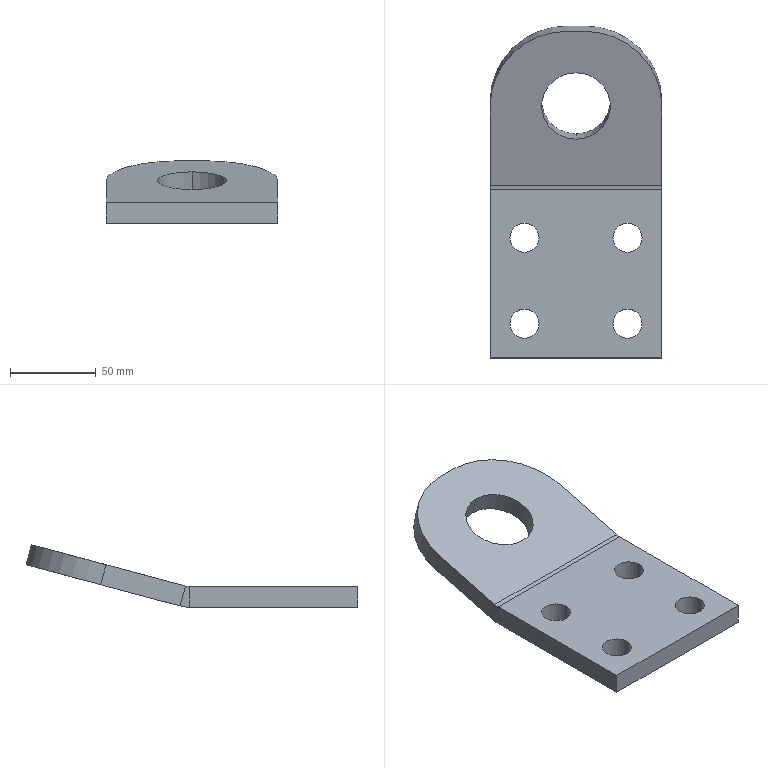Part | SolidWorks | 1 solid | 26 faces | box 100 x 193.34 x 36.386 mm | volume 197596 mm3 | cylinder 14 | plane 12 | commonest cylinder face diameters 17 x8 40 x2 90 x2 20 x1 44 x1
STEP:
#1=CARTESIAN_POINT('',(-38.5,-27.5,-12.));
#2=VERTEX_POINT('',#1);
#3=CARTESIAN_POINT('',(-21.5,-27.5,-12.));
#4=VERTEX_POINT('',#3);
#5=CARTESIAN_POINT('',(-30.,-27.5,-12.));
#6=DIRECTION('',(0.,0.,1.));
#7=DIRECTION('',(-1.,0.,0.));
#8=AXIS2_PLACEMENT_3D('',#5,#6,#7);
#9=CIRCLE('',#8,8.5);
#10=EDGE_CURVE('',#2,#4,#9,.T.);
#11=ORIENTED_EDGE('',*,*,#10,.F.);
#12=CARTESIAN_POINT('',(-38.5,-27.5,0.));
#13=VERTEX_POINT('',#12);
#14=CARTESIAN_POINT('',(-38.5,-27.5,-12.001));
#15=DIRECTION('',(0.,0.,1.));
#16=VECTOR('',#15,1000.);
#17=LINE('',#14,#16);
#18=EDGE_CURVE('',#2,#13,#17,.T.);
#19=ORIENTED_EDGE('',*,*,#18,.T.);
#20=CARTESIAN_POINT('',(-21.5,-27.5,0.));
#21=VERTEX_POINT('',#20);
#22=CARTESIAN_POINT('',(-30.,-27.5,0.));
#23=DIRECTION('',(0.,0.,1.));
#24=DIRECTION('',(1.,0.,0.));
#25=AXIS2_PLACEMENT_3D('',#22,#23,#24);
#26=CIRCLE('',#25,8.5);
#27=EDGE_CURVE('',#13,#21,#26,.T.);
#28=ORIENTED_EDGE('',*,*,#27,.T.);
#29=CARTESIAN_POINT('',(-21.5,-27.5,-12.001));
#30=DIRECTION('',(0.,0.,1.));
#31=VECTOR('',#30,1000.);
#32=LINE('',#29,#31);
#33=EDGE_CURVE('',#4,#21,#32,.T.);
#34=ORIENTED_EDGE('',*,*,#33,.F.);
#35=EDGE_LOOP('',(#11,#19,#28,#34));
#36=FACE_OUTER_BOUND('',#35,.T.);
#37=CARTESIAN_POINT('',(-30.,-27.5,-12.001));
#38=DIRECTION('',(0.,0.,1.));
#39=DIRECTION('',(1.,0.,0.));
#40=AXIS2_PLACEMENT_3D('',#37,#38,#39);
#41=CYLINDRICAL_SURFACE('',#40,8.5);
#42=ADVANCED_FACE('',(#36),#41,.F.);
#43=CARTESIAN_POINT('',(21.5,-27.5,-12.));
#44=VERTEX_POINT('',#43);
#45=CARTESIAN_POINT('',(38.5,-27.5,-12.));
#46=VERTEX_POINT('',#45);
#47=CARTESIAN_POINT('',(30.,-27.5,-12.));
#48=DIRECTION('',(0.,0.,1.));
#49=DIRECTION('',(-1.,0.,0.));
#50=AXIS2_PLACEMENT_3D('',#47,#48,#49);
#51=CIRCLE('',#50,8.5);
#52=EDGE_CURVE('',#44,#46,#51,.T.);
#53=ORIENTED_EDGE('',*,*,#52,.F.);
#54=CARTESIAN_POINT('',(21.5,-27.5,0.));
#55=VERTEX_POINT('',#54);
#56=CARTESIAN_POINT('',(21.5,-27.5,-12.001));
#57=DIRECTION('',(0.,0.,1.));
#58=VECTOR('',#57,1000.);
#59=LINE('',#56,#58);
#60=EDGE_CURVE('',#44,#55,#59,.T.);
#61=ORIENTED_EDGE('',*,*,#60,.T.);
#62=CARTESIAN_POINT('',(38.5,-27.5,0.));
#63=VERTEX_POINT('',#62);
#64=CARTESIAN_POINT('',(30.,-27.5,0.));
#65=DIRECTION('',(0.,0.,1.));
#66=DIRECTION('',(1.,0.,0.));
#67=AXIS2_PLACEMENT_3D('',#64,#65,#66);
#68=CIRCLE('',#67,8.5);
#69=EDGE_CURVE('',#55,#63,#68,.T.);
#70=ORIENTED_EDGE('',*,*,#69,.T.);
#71=CARTESIAN_POINT('',(38.5,-27.5,-12.001));
#72=DIRECTION('',(0.,0.,1.));
#73=VECTOR('',#72,1000.);
#74=LINE('',#71,#73);
#75=EDGE_CURVE('',#46,#63,#74,.T.);
#76=ORIENTED_EDGE('',*,*,#75,.F.);
#77=EDGE_LOOP('',(#53,#61,#70,#76));
#78=FACE_OUTER_BOUND('',#77,.T.);
#79=CARTESIAN_POINT('',(30.,-27.5,-12.001));
#80=DIRECTION('',(0.,0.,1.));
#81=DIRECTION('',(1.,0.,0.));
#82=AXIS2_PLACEMENT_3D('',#79,#80,#81);
#83=CYLINDRICAL_SURFACE('',#82,8.5);
#84=ADVANCED_FACE('',(#78),#83,.F.);
#85=CARTESIAN_POINT('',(21.5,-77.5,-12.));
#86=VERTEX_POINT('',#85);
#87=CARTESIAN_POINT('',(38.5,-77.5,-12.));
#88=VERTEX_POINT('',#87);
#89=CARTESIAN_POINT('',(30.,-77.5,-12.));
#90=DIRECTION('',(0.,0.,1.));
#91=DIRECTION('',(-1.,0.,0.));
#92=AXIS2_PLACEMENT_3D('',#89,#90,#91);
#93=CIRCLE('',#92,8.5);
#94=EDGE_CURVE('',#86,#88,#93,.T.);
#95=ORIENTED_EDGE('',*,*,#94,.F.);
#96=CARTESIAN_POINT('',(21.5,-77.5,0.));
#97=VERTEX_POINT('',#96);
#98=CARTESIAN_POINT('',(21.5,-77.5,-12.001));
#99=DIRECTION('',(0.,0.,1.));
#100=VECTOR('',#99,1000.);
#101=LINE('',#98,#100);
#102=EDGE_CURVE('',#86,#97,#101,.T.);
#103=ORIENTED_EDGE('',*,*,#102,.T.);
#104=CARTESIAN_POINT('',(38.5,-77.5,0.));
#105=VERTEX_POINT('',#104);
#106=CARTESIAN_POINT('',(30.,-77.5,0.));
#107=DIRECTION('',(0.,0.,1.));
#108=DIRECTION('',(1.,0.,0.));
#109=AXIS2_PLACEMENT_3D('',#106,#107,#108);
#110=CIRCLE('',#109,8.5);
#111=EDGE_CURVE('',#97,#105,#110,.T.);
#112=ORIENTED_EDGE('',*,*,#111,.T.);
#113=CARTESIAN_POINT('',(38.5,-77.5,-12.001));
#114=DIRECTION('',(0.,0.,1.));
#115=VECTOR('',#114,1000.);
#116=LINE('',#113,#115);
#117=EDGE_CURVE('',#88,#105,#116,.T.);
#118=ORIENTED_EDGE('',*,*,#117,.F.);
#119=EDGE_LOOP('',(#95,#103,#112,#118));
#120=FACE_OUTER_BOUND('',#119,.T.);
#121=CARTESIAN_POINT('',(30.,-77.5,-12.001));
#122=DIRECTION('',(0.,0.,1.));
#123=DIRECTION('',(1.,0.,0.));
#124=AXIS2_PLACEMENT_3D('',#121,#122,#123);
#125=CYLINDRICAL_SURFACE('',#124,8.5);
#126=ADVANCED_FACE('',(#120),#125,.F.);
#127=CARTESIAN_POINT('',(-38.5,-77.5,-12.));
#128=VERTEX_POINT('',#127);
#129=CARTESIAN_POINT('',(-21.5,-77.5,-12.));
#130=VERTEX_POINT('',#129);
#131=CARTESIAN_POINT('',(-30.,-77.5,-12.));
#132=DIRECTION('',(0.,0.,1.));
#133=DIRECTION('',(-1.,0.,0.));
#134=AXIS2_PLACEMENT_3D('',#131,#132,#133);
#135=CIRCLE('',#134,8.5);
#136=EDGE_CURVE('',#128,#130,#135,.T.);
#137=ORIENTED_EDGE('',*,*,#136,.F.);
#138=CARTESIAN_POINT('',(-38.5,-77.5,0.));
#139=VERTEX_POINT('',#138);
#140=CARTESIAN_POINT('',(-38.5,-77.5,-12.001));
#141=DIRECTION('',(0.,0.,1.));
#142=VECTOR('',#141,1000.);
#143=LINE('',#140,#142);
#144=EDGE_CURVE('',#128,#139,#143,.T.);
#145=ORIENTED_EDGE('',*,*,#144,.T.);
#146=CARTESIAN_POINT('',(-21.5,-77.5,0.));
#147=VERTEX_POINT('',#146);
#148=CARTESIAN_POINT('',(-30.,-77.5,0.));
#149=DIRECTION('',(0.,0.,1.));
#150=DIRECTION('',(1.,0.,0.));
#151=AXIS2_PLACEMENT_3D('',#148,#149,#150);
#152=CIRCLE('',#151,8.5);
#153=EDGE_CURVE('',#139,#147,#152,.T.);
#154=ORIENTED_EDGE('',*,*,#153,.T.);
#155=CARTESIAN_POINT('',(-21.5,-77.5,-12.001));
#156=DIRECTION('',(0.,0.,1.));
#157=VECTOR('',#156,1000.);
#158=LINE('',#155,#157);
#159=EDGE_CURVE('',#130,#147,#158,.T.);
#160=ORIENTED_EDGE('',*,*,#159,.F.);
#161=EDGE_LOOP('',(#137,#145,#154,#160));
#162=FACE_OUTER_BOUND('',#161,.T.);
#163=CARTESIAN_POINT('',(-30.,-77.5,-12.001));
#164=DIRECTION('',(0.,0.,1.));
#165=DIRECTION('',(1.,0.,0.));
#166=AXIS2_PLACEMENT_3D('',#163,#164,#165);
#167=CYLINDRICAL_SURFACE('',#166,8.5);
#168=ADVANCED_FACE('',(#162),#167,.F.);
#169=CARTESIAN_POINT('',(0.,68.586,17.916));
#170=VERTEX_POINT('',#169);
#171=CARTESIAN_POINT('',(0.,29.949,7.563));
#172=VERTEX_POINT('',#171);
#173=CARTESIAN_POINT('',(0.,49.267,12.74));
#174=DIRECTION('',(0.,-0.2588,0.9659));
#175=DIRECTION('',(0.,0.9659,0.2588));
#176=AXIS2_PLACEMENT_3D('',#173,#174,#175);
#177=CIRCLE('',#176,20.);
#178=EDGE_CURVE('',#170,#172,#177,.T.);
#179=ORIENTED_EDGE('',*,*,#178,.T.);
#180=CARTESIAN_POINT('',(0.,33.054,-4.028));
#181=VERTEX_POINT('',#180);
#182=CARTESIAN_POINT('',(0.,17.205,55.123));
#183=DIRECTION('',(0.,0.2588,-0.9659));
#184=VECTOR('',#183,1000.);
#185=LINE('',#182,#184);
#186=EDGE_CURVE('',#172,#181,#185,.T.);
#187=ORIENTED_EDGE('',*,*,#186,.T.);
#188=CARTESIAN_POINT('',(0.,71.691,6.325));
#189=VERTEX_POINT('',#188);
#190=CARTESIAN_POINT('',(0.,52.373,1.149));
#191=DIRECTION('',(0.,0.2588,-0.9659));
#192=DIRECTION('',(0.,0.9659,0.2588));
#193=AXIS2_PLACEMENT_3D('',#190,#191,#192);
#194=CIRCLE('',#193,20.);
#195=EDGE_CURVE('',#181,#189,#194,.T.);
#196=ORIENTED_EDGE('',*,*,#195,.T.);
#197=CARTESIAN_POINT('',(0.,55.842,65.476));
#198=DIRECTION('',(0.,0.2588,-0.9659));
#199=VECTOR('',#198,1000.);
#200=LINE('',#197,#199);
#201=EDGE_CURVE('',#170,#189,#200,.T.);
#202=ORIENTED_EDGE('',*,*,#201,.F.);
#203=EDGE_LOOP('',(#179,#187,#196,#202));
#204=FACE_OUTER_BOUND('',#203,.T.);
#205=CARTESIAN_POINT('',(0.,36.523,60.299));
#206=DIRECTION('',(0.,0.2588,-0.9659));
#207=DIRECTION('',(0.,0.9659,0.2588));
#208=AXIS2_PLACEMENT_3D('',#205,#206,#207);
#209=CYLINDRICAL_SURFACE('',#208,20.);
#210=ADVANCED_FACE('',(#204),#209,.F.);
#211=ORIENTED_EDGE('',*,*,#178,.F.);
#212=CARTESIAN_POINT('',(0.,49.267,12.74));
#213=DIRECTION('',(0.,-0.2588,0.9659));
#214=DIRECTION('',(0.,0.9659,0.2588));
#215=AXIS2_PLACEMENT_3D('',#212,#213,#214);
#216=CIRCLE('',#215,20.);
#217=EDGE_CURVE('',#172,#170,#216,.T.);
#218=ORIENTED_EDGE('',*,*,#217,.F.);
#219=EDGE_LOOP('',(#211,#218));
#220=FACE_BOUND('',#219,.T.);
#221=CARTESIAN_POINT('',(5.,92.734,24.386));
#222=VERTEX_POINT('',#221);
#223=CARTESIAN_POINT('',(-5.,92.734,24.386));
#224=VERTEX_POINT('',#223);
#225=CARTESIAN_POINT('',(-50.,92.734,24.386));
#226=DIRECTION('',(-1.,0.,0.));
#227=VECTOR('',#226,1000.);
#228=LINE('',#225,#227);
#229=EDGE_CURVE('',#222,#224,#228,.T.);
#230=ORIENTED_EDGE('',*,*,#229,.T.);
#231=CARTESIAN_POINT('',(-50.,49.267,12.74));
#232=VERTEX_POINT('',#231);
#233=CARTESIAN_POINT('',(-5.,49.267,12.74));
#234=DIRECTION('',(0.,-0.2588,0.9659));
#235=DIRECTION('',(0.,0.9659,0.2588));
#236=AXIS2_PLACEMENT_3D('',#233,#234,#235);
#237=CIRCLE('',#236,45.);
#238=EDGE_CURVE('',#224,#232,#237,.T.);
#239=ORIENTED_EDGE('',*,*,#238,.T.);
#240=CARTESIAN_POINT('',(-50.,2.994,0.3407));
#241=VERTEX_POINT('',#240);
#242=CARTESIAN_POINT('',(-50.,-95.622,-26.083));
#243=DIRECTION('',(0.,-0.9659,-0.2588));
#244=VECTOR('',#243,1000.);
#245=LINE('',#242,#244);
#246=EDGE_CURVE('',#232,#241,#245,.T.);
#247=ORIENTED_EDGE('',*,*,#246,.T.);
#248=CARTESIAN_POINT('',(50.,2.994,0.3407));
#249=VERTEX_POINT('',#248);
#250=CARTESIAN_POINT('',(0.,2.994,0.3407));
#251=DIRECTION('',(1.,0.,0.));
#252=VECTOR('',#251,1000.);
#253=LINE('',#250,#252);
#254=EDGE_CURVE('',#241,#249,#253,.T.);
#255=ORIENTED_EDGE('',*,*,#254,.T.);
#256=CARTESIAN_POINT('',(50.,49.267,12.74));
#257=VERTEX_POINT('',#256);
#258=CARTESIAN_POINT('',(50.,-95.622,-26.083));
#259=DIRECTION('',(0.,0.9659,0.2588));
#260=VECTOR('',#259,1000.);
#261=LINE('',#258,#260);
#262=EDGE_CURVE('',#249,#257,#261,.T.);
#263=ORIENTED_EDGE('',*,*,#262,.T.);
#264=CARTESIAN_POINT('',(5.,49.267,12.74));
#265=DIRECTION('',(0.,-0.2588,0.9659));
#266=DIRECTION('',(0.,0.9659,0.2588));
#267=AXIS2_PLACEMENT_3D('',#264,#265,#266);
#268=CIRCLE('',#267,45.);
#269=EDGE_CURVE('',#257,#222,#268,.T.);
#270=ORIENTED_EDGE('',*,*,#269,.T.);
#271=EDGE_LOOP('',(#230,#239,#247,#255,#263,#270));
#272=FACE_OUTER_BOUND('',#271,.T.);
#273=CARTESIAN_POINT('',(0.,-1.444,-0.8484));
#274=DIRECTION('',(0.,0.2588,-0.9659));
#275=DIRECTION('',(-1.,0.,0.));
#276=AXIS2_PLACEMENT_3D('',#273,#274,#275);
#277=PLANE('',#276);
#278=ADVANCED_FACE('',(#220,#272),#277,.F.);
#279=CARTESIAN_POINT('',(50.,6.1,-11.25));
#280=VERTEX_POINT('',#279);
#281=CARTESIAN_POINT('',(50.,52.373,1.149));
#282=VERTEX_POINT('',#281);
#283=CARTESIAN_POINT('',(50.,-92.516,-37.674));
#284=DIRECTION('',(0.,0.9659,0.2588));
#285=VECTOR('',#284,1000.);
#286=LINE('',#283,#285);
#287=EDGE_CURVE('',#280,#282,#286,.T.);
#288=ORIENTED_EDGE('',*,*,#287,.T.);
#289=CARTESIAN_POINT('',(50.,52.373,1.149));
#290=DIRECTION('',(0.,-0.2588,0.9659));
#291=VECTOR('',#290,1000.);
#292=LINE('',#289,#291);
#293=EDGE_CURVE('',#282,#257,#292,.T.);
#294=ORIENTED_EDGE('',*,*,#293,.T.);
#295=ORIENTED_EDGE('',*,*,#262,.F.);
#296=CARTESIAN_POINT('',(50.,6.1,-11.25));
#297=DIRECTION('',(0.,-0.2588,0.9659));
#298=VECTOR('',#297,1000.);
#299=LINE('',#296,#298);
#300=EDGE_CURVE('',#280,#249,#299,.T.);
#301=ORIENTED_EDGE('',*,*,#300,.F.);
#302=EDGE_LOOP('',(#288,#294,#295,#301));
#303=FACE_OUTER_BOUND('',#302,.T.);
#304=CARTESIAN_POINT('',(50.,-92.516,-37.674));
#305=DIRECTION('',(1.,0.,0.));
#306=DIRECTION('',(0.,0.2588,-0.9659));
#307=AXIS2_PLACEMENT_3D('',#304,#305,#306);
#308=PLANE('',#307);
#309=ADVANCED_FACE('',(#303),#308,.T.);
#310=ORIENTED_EDGE('',*,*,#246,.F.);
#311=CARTESIAN_POINT('',(-50.,52.373,1.149));
#312=VERTEX_POINT('',#311);
#313=CARTESIAN_POINT('',(-50.,52.373,1.149));
#314=DIRECTION('',(0.,0.2588,-0.9659));
#315=VECTOR('',#314,1000.);
#316=LINE('',#313,#315);
#317=EDGE_CURVE('',#232,#312,#316,.T.);
#318=ORIENTED_EDGE('',*,*,#317,.T.);
#319=CARTESIAN_POINT('',(-50.,6.1,-11.25));
#320=VERTEX_POINT('',#319);
#321=CARTESIAN_POINT('',(-50.,-92.516,-37.674));
#322=DIRECTION('',(0.,-0.9659,-0.2588));
#323=VECTOR('',#322,1000.);
#324=LINE('',#321,#323);
#325=EDGE_CURVE('',#312,#320,#324,.T.);
#326=ORIENTED_EDGE('',*,*,#325,.T.);
#327=CARTESIAN_POINT('',(-50.,6.1,-11.25));
#328=DIRECTION('',(0.,0.2588,-0.9659));
#329=VECTOR('',#328,1000.);
#330=LINE('',#327,#329);
#331=EDGE_CURVE('',#241,#320,#330,.T.);
#332=ORIENTED_EDGE('',*,*,#331,.F.);
#333=EDGE_LOOP('',(#310,#318,#326,#332));
#334=FACE_OUTER_BOUND('',#333,.T.);
#335=CARTESIAN_POINT('',(-50.,-92.516,-37.674));
#336=DIRECTION('',(-1.,0.,0.));
#337=DIRECTION('',(0.,-0.2588,0.9659));
#338=AXIS2_PLACEMENT_3D('',#335,#336,#337);
#339=PLANE('',#338);
#340=ADVANCED_FACE('',(#334),#339,.T.);
#341=CARTESIAN_POINT('',(5.,95.84,12.795));
#342=VERTEX_POINT('',#341);
#343=CARTESIAN_POINT('',(-5.,95.84,12.795));
#344=VERTEX_POINT('',#343);
#345=CARTESIAN_POINT('',(-50.,95.84,12.795));
#346=DIRECTION('',(-1.,0.,0.));
#347=VECTOR('',#346,1000.);
#348=LINE('',#345,#347);
#349=EDGE_CURVE('',#342,#344,#348,.T.);
#350=ORIENTED_EDGE('',*,*,#349,.T.);
#351=CARTESIAN_POINT('',(-5.,95.84,12.795));
#352=DIRECTION('',(0.,-0.2588,0.9659));
#353=VECTOR('',#352,1000.);
#354=LINE('',#351,#353);
#355=EDGE_CURVE('',#344,#224,#354,.T.);
#356=ORIENTED_EDGE('',*,*,#355,.T.);
#357=ORIENTED_EDGE('',*,*,#229,.F.);
#358=CARTESIAN_POINT('',(5.,95.84,12.795));
#359=DIRECTION('',(0.,0.2588,-0.9659));
#360=VECTOR('',#359,1000.);
#361=LINE('',#358,#360);
#362=EDGE_CURVE('',#222,#342,#361,.T.);
#363=ORIENTED_EDGE('',*,*,#362,.T.);
#364=EDGE_LOOP('',(#350,#356,#357,#363));
#365=FACE_OUTER_BOUND('',#364,.T.);
#366=CARTESIAN_POINT('',(-50.,95.84,12.795));
#367=DIRECTION('',(0.,0.9659,0.2588));
#368=DIRECTION('',(0.,-0.2588,0.9659));
#369=AXIS2_PLACEMENT_3D('',#366,#367,#368);
#370=PLANE('',#369);
#371=ADVANCED_FACE('',(#365),#370,.T.);
#372=CARTESIAN_POINT('',(0.,52.373,1.149));
#373=DIRECTION('',(0.,0.2588,-0.9659));
#374=DIRECTION('',(0.,0.9659,0.2588));
#375=AXIS2_PLACEMENT_3D('',#372,#373,#374);
#376=CIRCLE('',#375,20.);
#377=EDGE_CURVE('',#189,#181,#376,.T.);
#378=ORIENTED_EDGE('',*,*,#377,.F.);
#379=ORIENTED_EDGE('',*,*,#195,.F.);
#380=EDGE_LOOP('',(#378,#379));
#381=FACE_BOUND('',#380,.T.);
#382=ORIENTED_EDGE('',*,*,#325,.F.);
#383=CARTESIAN_POINT('',(-5.,52.373,1.149));
#384=DIRECTION('',(0.,0.2588,-0.9659));
#385=DIRECTION('',(0.,0.9659,0.2588));
#386=AXIS2_PLACEMENT_3D('',#383,#384,#385);
#387=CIRCLE('',#386,45.);
#388=EDGE_CURVE('',#312,#344,#387,.T.);
#389=ORIENTED_EDGE('',*,*,#388,.T.);
#390=ORIENTED_EDGE('',*,*,#349,.F.);
#391=CARTESIAN_POINT('',(5.,52.373,1.149));
#392=DIRECTION('',(0.,0.2588,-0.9659));
#393=DIRECTION('',(0.,0.9659,0.2588));
#394=AXIS2_PLACEMENT_3D('',#391,#392,#393);
#395=CIRCLE('',#394,45.);
#396=EDGE_CURVE('',#342,#282,#395,.T.);
#397=ORIENTED_EDGE('',*,*,#396,.T.);
#398=ORIENTED_EDGE('',*,*,#287,.F.);
#399=CARTESIAN_POINT('',(0.,6.1,-11.25));
#400=DIRECTION('',(1.,0.,0.));
#401=VECTOR('',#400,1000.);
#402=LINE('',#399,#401);
#403=EDGE_CURVE('',#320,#280,#402,.T.);
#404=ORIENTED_EDGE('',*,*,#403,.F.);
#405=EDGE_LOOP('',(#382,#389,#390,#397,#398,#404));
#406=FACE_OUTER_BOUND('',#405,.T.);
#407=CARTESIAN_POINT('',(0.,1.662,-12.439));
#408=DIRECTION('',(0.,0.2588,-0.9659));
#409=DIRECTION('',(-1.,0.,0.));
#410=AXIS2_PLACEMENT_3D('',#407,#408,#409);
#411=PLANE('',#410);
#412=ADVANCED_FACE('',(#381,#406),#411,.T.);
#413=CARTESIAN_POINT('',(-50.,-97.5,0.));
#414=VERTEX_POINT('',#413);
#415=CARTESIAN_POINT('',(50.,-97.5,0.));
#416=VERTEX_POINT('',#415);
#417=CARTESIAN_POINT('',(-50.,-97.5,0.));
#418=DIRECTION('',(1.,0.,0.));
#419=VECTOR('',#418,1000.);
#420=LINE('',#417,#419);
#421=EDGE_CURVE('',#414,#416,#420,.T.);
#422=ORIENTED_EDGE('',*,*,#421,.F.);
#423=CARTESIAN_POINT('',(-50.,-97.5,-12.));
#424=VERTEX_POINT('',#423);
#425=CARTESIAN_POINT('',(-50.,-97.5,-12.));
#426=DIRECTION('',(0.,0.,1.));
#427=VECTOR('',#426,1000.);
#428=LINE('',#425,#427);
#429=EDGE_CURVE('',#424,#414,#428,.T.);
#430=ORIENTED_EDGE('',*,*,#429,.F.);
#431=CARTESIAN_POINT('',(50.,-97.5,-12.));
#432=VERTEX_POINT('',#431);
#433=CARTESIAN_POINT('',(-50.,-97.5,-12.));
#434=DIRECTION('',(1.,0.,0.));
#435=VECTOR('',#434,1000.);
#436=LINE('',#433,#435);
#437=EDGE_CURVE('',#424,#432,#436,.T.);
#438=ORIENTED_EDGE('',*,*,#437,.T.);
#439=CARTESIAN_POINT('',(50.,-97.5,-12.));
#440=DIRECTION('',(0.,0.,1.));
#441=VECTOR('',#440,1000.);
#442=LINE('',#439,#441);
#443=EDGE_CURVE('',#432,#416,#442,.T.);
#444=ORIENTED_EDGE('',*,*,#443,.T.);
#445=EDGE_LOOP('',(#422,#430,#438,#444));
#446=FACE_OUTER_BOUND('',#445,.T.);
#447=CARTESIAN_POINT('',(-50.,-97.5,-12.));
#448=DIRECTION('',(0.,-1.,0.));
#449=DIRECTION('',(0.,0.,-1.));
#450=AXIS2_PLACEMENT_3D('',#447,#448,#449);
#451=PLANE('',#450);
#452=ADVANCED_FACE('',(#446),#451,.T.);
#453=CARTESIAN_POINT('',(-30.,-27.5,-12.));
#454=DIRECTION('',(0.,0.,1.));
#455=DIRECTION('',(-1.,0.,0.));
#456=AXIS2_PLACEMENT_3D('',#453,#454,#455);
#457=CIRCLE('',#456,8.5);
#458=EDGE_CURVE('',#4,#2,#457,.T.);
#459=ORIENTED_EDGE('',*,*,#458,.T.);
#460=ORIENTED_EDGE('',*,*,#10,.T.);
#461=EDGE_LOOP('',(#459,#460));
#462=FACE_BOUND('',#461,.T.);
#463=CARTESIAN_POINT('',(30.,-27.5,-12.));
#464=DIRECTION('',(0.,0.,1.));
#465=DIRECTION('',(-1.,0.,0.));
#466=AXIS2_PLACEMENT_3D('',#463,#464,#465);
#467=CIRCLE('',#466,8.5);
#468=EDGE_CURVE('',#46,#44,#467,.T.);
#469=ORIENTED_EDGE('',*,*,#468,.T.);
#470=ORIENTED_EDGE('',*,*,#52,.T.);
#471=EDGE_LOOP('',(#469,#470));
#472=FACE_BOUND('',#471,.T.);
#473=CARTESIAN_POINT('',(30.,-77.5,-12.));
#474=DIRECTION('',(0.,0.,1.));
#475=DIRECTION('',(-1.,0.,0.));
#476=AXIS2_PLACEMENT_3D('',#473,#474,#475);
#477=CIRCLE('',#476,8.5);
#478=EDGE_CURVE('',#88,#86,#477,.T.);
#479=ORIENTED_EDGE('',*,*,#478,.T.);
#480=ORIENTED_EDGE('',*,*,#94,.T.);
#481=EDGE_LOOP('',(#479,#480));
#482=FACE_BOUND('',#481,.T.);
#483=CARTESIAN_POINT('',(-30.,-77.5,-12.));
#484=DIRECTION('',(0.,0.,1.));
#485=DIRECTION('',(-1.,0.,0.));
#486=AXIS2_PLACEMENT_3D('',#483,#484,#485);
#487=CIRCLE('',#486,8.5);
#488=EDGE_CURVE('',#130,#128,#487,.T.);
#489=ORIENTED_EDGE('',*,*,#488,.T.);
#490=ORIENTED_EDGE('',*,*,#136,.T.);
#491=EDGE_LOOP('',(#489,#490));
#492=FACE_BOUND('',#491,.T.);
#493=CARTESIAN_POINT('',(-50.,0.4056,-12.));
#494=VERTEX_POINT('',#493);
#495=CARTESIAN_POINT('',(-50.,-97.5,-12.));
#496=DIRECTION('',(0.,-1.,0.));
#497=VECTOR('',#496,1000.);
#498=LINE('',#495,#497);
#499=EDGE_CURVE('',#494,#424,#498,.T.);
#500=ORIENTED_EDGE('',*,*,#499,.F.);
#501=CARTESIAN_POINT('',(50.,0.4056,-12.));
#502=VERTEX_POINT('',#501);
#503=CARTESIAN_POINT('',(0.,0.4056,-12.));
#504=DIRECTION('',(1.,0.,0.));
#505=VECTOR('',#504,1000.);
#506=LINE('',#503,#505);
#507=EDGE_CURVE('',#494,#502,#506,.T.);
#508=ORIENTED_EDGE('',*,*,#507,.T.);
#509=CARTESIAN_POINT('',(50.,-97.5,-12.));
#510=DIRECTION('',(0.,1.,0.));
#511=VECTOR('',#510,1000.);
#512=LINE('',#509,#511);
#513=EDGE_CURVE('',#432,#502,#512,.T.);
#514=ORIENTED_EDGE('',*,*,#513,.F.);
#515=ORIENTED_EDGE('',*,*,#437,.F.);
#516=EDGE_LOOP('',(#500,#508,#514,#515));
#517=FACE_OUTER_BOUND('',#516,.T.);
#518=CARTESIAN_POINT('',(0.,0.,-12.));
#519=DIRECTION('',(0.,0.,-1.));
#520=DIRECTION('',(-1.,0.,0.));
#521=AXIS2_PLACEMENT_3D('',#518,#519,#520);
#522=PLANE('',#521);
#523=ADVANCED_FACE('',(#462,#472,#482,#492,#517),#522,.T.);
#524=ORIENTED_EDGE('',*,*,#513,.T.);
#525=CARTESIAN_POINT('',(50.,0.4056,0.));
#526=VERTEX_POINT('',#525);
#527=CARTESIAN_POINT('',(50.,0.4056,-12.));
#528=DIRECTION('',(0.,0.,1.));
#529=VECTOR('',#528,1000.);
#530=LINE('',#527,#529);
#531=EDGE_CURVE('',#502,#526,#530,.T.);
#532=ORIENTED_EDGE('',*,*,#531,.T.);
#533=CARTESIAN_POINT('',(50.,-97.5,0.));
#534=DIRECTION('',(0.,1.,0.));
#535=VECTOR('',#534,1000.);
#536=LINE('',#533,#535);
#537=EDGE_CURVE('',#416,#526,#536,.T.);
#538=ORIENTED_EDGE('',*,*,#537,.F.);
#539=ORIENTED_EDGE('',*,*,#443,.F.);
#540=EDGE_LOOP('',(#524,#532,#538,#539));
#541=FACE_OUTER_BOUND('',#540,.T.);
#542=CARTESIAN_POINT('',(50.,-97.5,-12.));
#543=DIRECTION('',(1.,0.,0.));
#544=DIRECTION('',(0.,0.,-1.));
#545=AXIS2_PLACEMENT_3D('',#542,#543,#544);
#546=PLANE('',#545);
#547=ADVANCED_FACE('',(#541),#546,.T.);
#548=CARTESIAN_POINT('',(-30.,-27.5,0.));
#549=DIRECTION('',(0.,0.,1.));
#550=DIRECTION('',(1.,0.,0.));
#551=AXIS2_PLACEMENT_3D('',#548,#549,#550);
#552=CIRCLE('',#551,8.5);
#553=EDGE_CURVE('',#21,#13,#552,.T.);
#554=ORIENTED_EDGE('',*,*,#553,.F.);
#555=ORIENTED_EDGE('',*,*,#27,.F.);
#556=EDGE_LOOP('',(#554,#555));
#557=FACE_BOUND('',#556,.T.);
#558=CARTESIAN_POINT('',(30.,-27.5,0.));
#559=DIRECTION('',(0.,0.,1.));
#560=DIRECTION('',(1.,0.,0.));
#561=AXIS2_PLACEMENT_3D('',#558,#559,#560);
#562=CIRCLE('',#561,8.5);
#563=EDGE_CURVE('',#63,#55,#562,.T.);
#564=ORIENTED_EDGE('',*,*,#563,.F.);
#565=ORIENTED_EDGE('',*,*,#69,.F.);
#566=EDGE_LOOP('',(#564,#565));
#567=FACE_BOUND('',#566,.T.);
#568=CARTESIAN_POINT('',(30.,-77.5,0.));
#569=DIRECTION('',(0.,0.,1.));
#570=DIRECTION('',(1.,0.,0.));
#571=AXIS2_PLACEMENT_3D('',#568,#569,#570);
#572=CIRCLE('',#571,8.5);
#573=EDGE_CURVE('',#105,#97,#572,.T.);
#574=ORIENTED_EDGE('',*,*,#573,.F.);
#575=ORIENTED_EDGE('',*,*,#111,.F.);
#576=EDGE_LOOP('',(#574,#575));
#577=FACE_BOUND('',#576,.T.);
#578=CARTESIAN_POINT('',(-30.,-77.5,0.));
#579=DIRECTION('',(0.,0.,1.));
#580=DIRECTION('',(1.,0.,0.));
#581=AXIS2_PLACEMENT_3D('',#578,#579,#580);
#582=CIRCLE('',#581,8.5);
#583=EDGE_CURVE('',#147,#139,#582,.T.);
#584=ORIENTED_EDGE('',*,*,#583,.F.);
#585=ORIENTED_EDGE('',*,*,#153,.F.);
#586=EDGE_LOOP('',(#584,#585));
#587=FACE_BOUND('',#586,.T.);
#588=CARTESIAN_POINT('',(-50.,0.4056,0.));
#589=VERTEX_POINT('',#588);
#590=CARTESIAN_POINT('',(0.,0.4056,0.));
#591=DIRECTION('',(1.,0.,0.));
#592=VECTOR('',#591,1000.);
#593=LINE('',#590,#592);
#594=EDGE_CURVE('',#589,#526,#593,.T.);
#595=ORIENTED_EDGE('',*,*,#594,.F.);
#596=CARTESIAN_POINT('',(-50.,-97.5,0.));
#597=DIRECTION('',(0.,-1.,0.));
#598=VECTOR('',#597,1000.);
#599=LINE('',#596,#598);
#600=EDGE_CURVE('',#589,#414,#599,.T.);
#601=ORIENTED_EDGE('',*,*,#600,.T.);
#602=ORIENTED_EDGE('',*,*,#421,.T.);
#603=ORIENTED_EDGE('',*,*,#537,.T.);
#604=EDGE_LOOP('',(#595,#601,#602,#603));
#605=FACE_OUTER_BOUND('',#604,.T.);
#606=CARTESIAN_POINT('',(0.,0.,0.));
#607=DIRECTION('',(0.,0.,-1.));
#608=DIRECTION('',(-1.,0.,0.));
#609=AXIS2_PLACEMENT_3D('',#606,#607,#608);
#610=PLANE('',#609);
#611=ADVANCED_FACE('',(#557,#567,#577,#587,#605),#610,.F.);
#612=ORIENTED_EDGE('',*,*,#600,.F.);
#613=CARTESIAN_POINT('',(-50.,0.4056,-12.));
#614=DIRECTION('',(0.,0.,-1.));
#615=VECTOR('',#614,1000.);
#616=LINE('',#613,#615);
#617=EDGE_CURVE('',#589,#494,#616,.T.);
#618=ORIENTED_EDGE('',*,*,#617,.T.);
#619=ORIENTED_EDGE('',*,*,#499,.T.);
#620=ORIENTED_EDGE('',*,*,#429,.T.);
#621=EDGE_LOOP('',(#612,#618,#619,#620));
#622=FACE_OUTER_BOUND('',#621,.T.);
#623=CARTESIAN_POINT('',(-50.,-97.5,-12.));
#624=DIRECTION('',(-1.,0.,0.));
#625=DIRECTION('',(0.,0.,1.));
#626=AXIS2_PLACEMENT_3D('',#623,#624,#625);
#627=PLANE('',#626);
#628=ADVANCED_FACE('',(#622),#627,.T.);
#629=ORIENTED_EDGE('',*,*,#617,.F.);
#630=CARTESIAN_POINT('',(-50.,0.4056,10.));
#631=DIRECTION('',(1.,0.,0.));
#632=DIRECTION('',(0.,0.,-1.));
#633=AXIS2_PLACEMENT_3D('',#630,#631,#632);
#634=CIRCLE('',#633,10.);
#635=EDGE_CURVE('',#589,#241,#634,.T.);
#636=ORIENTED_EDGE('',*,*,#635,.T.);
#637=ORIENTED_EDGE('',*,*,#331,.T.);
#638=CARTESIAN_POINT('',(-50.,0.4056,10.));
#639=DIRECTION('',(1.,0.,0.));
#640=DIRECTION('',(0.,0.,1.));
#641=AXIS2_PLACEMENT_3D('',#638,#639,#640);
#642=CIRCLE('',#641,22.);
#643=EDGE_CURVE('',#494,#320,#642,.T.);
#644=ORIENTED_EDGE('',*,*,#643,.F.);
#645=EDGE_LOOP('',(#629,#636,#637,#644));
#646=FACE_OUTER_BOUND('',#645,.T.);
#647=CARTESIAN_POINT('',(-50.,0.4056,10.));
#648=DIRECTION('',(-1.,0.,0.));
#649=DIRECTION('',(0.,0.,1.));
#650=AXIS2_PLACEMENT_3D('',#647,#648,#649);
#651=PLANE('',#650);
#652=ADVANCED_FACE('',(#646),#651,.T.);
#653=CARTESIAN_POINT('',(50.,0.4056,10.));
#654=DIRECTION('',(-1.,0.,0.));
#655=DIRECTION('',(0.,0.,-1.));
#656=AXIS2_PLACEMENT_3D('',#653,#654,#655);
#657=CIRCLE('',#656,10.);
#658=EDGE_CURVE('',#249,#526,#657,.T.);
#659=ORIENTED_EDGE('',*,*,#658,.T.);
#660=ORIENTED_EDGE('',*,*,#531,.F.);
#661=CARTESIAN_POINT('',(50.,0.4056,10.));
#662=DIRECTION('',(-1.,0.,0.));
#663=DIRECTION('',(0.,0.,-1.));
#664=AXIS2_PLACEMENT_3D('',#661,#662,#663);
#665=CIRCLE('',#664,22.);
#666=EDGE_CURVE('',#280,#502,#665,.T.);
#667=ORIENTED_EDGE('',*,*,#666,.F.);
#668=ORIENTED_EDGE('',*,*,#300,.T.);
#669=EDGE_LOOP('',(#659,#660,#667,#668));
#670=FACE_OUTER_BOUND('',#669,.T.);
#671=CARTESIAN_POINT('',(50.,0.4056,10.));
#672=DIRECTION('',(1.,0.,0.));
#673=DIRECTION('',(0.,0.,-1.));
#674=AXIS2_PLACEMENT_3D('',#671,#672,#673);
#675=PLANE('',#674);
#676=ADVANCED_FACE('',(#670),#675,.T.);
#677=ORIENTED_EDGE('',*,*,#403,.T.);
#678=ORIENTED_EDGE('',*,*,#666,.T.);
#679=ORIENTED_EDGE('',*,*,#507,.F.);
#680=ORIENTED_EDGE('',*,*,#643,.T.);
#681=EDGE_LOOP('',(#677,#678,#679,#680));
#682=FACE_OUTER_BOUND('',#681,.T.);
#683=CARTESIAN_POINT('',(-100.804,0.4056,10.));
#684=DIRECTION('',(1.,0.,0.));
#685=DIRECTION('',(0.,0.,-1.));
#686=AXIS2_PLACEMENT_3D('',#683,#684,#685);
#687=CYLINDRICAL_SURFACE('',#686,22.);
#688=ADVANCED_FACE('',(#682),#687,.T.);
#689=ORIENTED_EDGE('',*,*,#254,.F.);
#690=ORIENTED_EDGE('',*,*,#635,.F.);
#691=ORIENTED_EDGE('',*,*,#594,.T.);
#692=ORIENTED_EDGE('',*,*,#658,.F.);
#693=EDGE_LOOP('',(#689,#690,#691,#692));
#694=FACE_OUTER_BOUND('',#693,.T.);
#695=CARTESIAN_POINT('',(-100.804,0.4056,10.));
#696=DIRECTION('',(1.,0.,0.));
#697=DIRECTION('',(0.,0.,-1.));
#698=AXIS2_PLACEMENT_3D('',#695,#696,#697);
#699=CYLINDRICAL_SURFACE('',#698,10.);
#700=ADVANCED_FACE('',(#694),#699,.F.);
#701=ORIENTED_EDGE('',*,*,#186,.F.);
#702=ORIENTED_EDGE('',*,*,#217,.T.);
#703=ORIENTED_EDGE('',*,*,#201,.T.);
#704=ORIENTED_EDGE('',*,*,#377,.T.);
#705=EDGE_LOOP('',(#701,#702,#703,#704));
#706=FACE_OUTER_BOUND('',#705,.T.);
#707=CARTESIAN_POINT('',(0.,36.523,60.299));
#708=DIRECTION('',(0.,0.2588,-0.9659));
#709=DIRECTION('',(0.,0.9659,0.2588));
#710=AXIS2_PLACEMENT_3D('',#707,#708,#709);
#711=CYLINDRICAL_SURFACE('',#710,20.);
#712=ADVANCED_FACE('',(#706),#711,.F.);
#713=ORIENTED_EDGE('',*,*,#388,.F.);
#714=ORIENTED_EDGE('',*,*,#317,.F.);
#715=ORIENTED_EDGE('',*,*,#238,.F.);
#716=ORIENTED_EDGE('',*,*,#355,.F.);
#717=EDGE_LOOP('',(#713,#714,#715,#716));
#718=FACE_OUTER_BOUND('',#717,.T.);
#719=CARTESIAN_POINT('',(-5.,52.373,1.149));
#720=DIRECTION('',(0.,-0.2588,0.9659));
#721=DIRECTION('',(0.,-0.9659,-0.2588));
#722=AXIS2_PLACEMENT_3D('',#719,#720,#721);
#723=CYLINDRICAL_SURFACE('',#722,45.);
#724=ADVANCED_FACE('',(#718),#723,.T.);
#725=ORIENTED_EDGE('',*,*,#396,.F.);
#726=ORIENTED_EDGE('',*,*,#362,.F.);
#727=ORIENTED_EDGE('',*,*,#269,.F.);
#728=ORIENTED_EDGE('',*,*,#293,.F.);
#729=EDGE_LOOP('',(#725,#726,#727,#728));
#730=FACE_OUTER_BOUND('',#729,.T.);
#731=CARTESIAN_POINT('',(5.,52.373,1.149));
#732=DIRECTION('',(0.,-0.2588,0.9659));
#733=DIRECTION('',(0.,-0.9659,-0.2588));
#734=AXIS2_PLACEMENT_3D('',#731,#732,#733);
#735=CYLINDRICAL_SURFACE('',#734,45.);
#736=ADVANCED_FACE('',(#730),#735,.T.);
#737=ORIENTED_EDGE('',*,*,#144,.F.);
#738=ORIENTED_EDGE('',*,*,#488,.F.);
#739=ORIENTED_EDGE('',*,*,#159,.T.);
#740=ORIENTED_EDGE('',*,*,#583,.T.);
#741=EDGE_LOOP('',(#737,#738,#739,#740));
#742=FACE_OUTER_BOUND('',#741,.T.);
#743=CARTESIAN_POINT('',(-30.,-77.5,-12.001));
#744=DIRECTION('',(0.,0.,1.));
#745=DIRECTION('',(1.,0.,0.));
#746=AXIS2_PLACEMENT_3D('',#743,#744,#745);
#747=CYLINDRICAL_SURFACE('',#746,8.5);
#748=ADVANCED_FACE('',(#742),#747,.F.);
#749=ORIENTED_EDGE('',*,*,#102,.F.);
#750=ORIENTED_EDGE('',*,*,#478,.F.);
#751=ORIENTED_EDGE('',*,*,#117,.T.);
#752=ORIENTED_EDGE('',*,*,#573,.T.);
#753=EDGE_LOOP('',(#749,#750,#751,#752));
#754=FACE_OUTER_BOUND('',#753,.T.);
#755=CARTESIAN_POINT('',(30.,-77.5,-12.001));
#756=DIRECTION('',(0.,0.,1.));
#757=DIRECTION('',(1.,0.,0.));
#758=AXIS2_PLACEMENT_3D('',#755,#756,#757);
#759=CYLINDRICAL_SURFACE('',#758,8.5);
#760=ADVANCED_FACE('',(#754),#759,.F.);
#761=ORIENTED_EDGE('',*,*,#60,.F.);
#762=ORIENTED_EDGE('',*,*,#468,.F.);
#763=ORIENTED_EDGE('',*,*,#75,.T.);
#764=ORIENTED_EDGE('',*,*,#563,.T.);
#765=EDGE_LOOP('',(#761,#762,#763,#764));
#766=FACE_OUTER_BOUND('',#765,.T.);
#767=CARTESIAN_POINT('',(30.,-27.5,-12.001));
#768=DIRECTION('',(0.,0.,1.));
#769=DIRECTION('',(1.,0.,0.));
#770=AXIS2_PLACEMENT_3D('',#767,#768,#769);
#771=CYLINDRICAL_SURFACE('',#770,8.5);
#772=ADVANCED_FACE('',(#766),#771,.F.);
#773=ORIENTED_EDGE('',*,*,#18,.F.);
#774=ORIENTED_EDGE('',*,*,#458,.F.);
#775=ORIENTED_EDGE('',*,*,#33,.T.);
#776=ORIENTED_EDGE('',*,*,#553,.T.);
#777=EDGE_LOOP('',(#773,#774,#775,#776));
#778=FACE_OUTER_BOUND('',#777,.T.);
#779=CARTESIAN_POINT('',(-30.,-27.5,-12.001));
#780=DIRECTION('',(0.,0.,1.));
#781=DIRECTION('',(1.,0.,0.));
#782=AXIS2_PLACEMENT_3D('',#779,#780,#781);
#783=CYLINDRICAL_SURFACE('',#782,8.5);
#784=ADVANCED_FACE('',(#778),#783,.F.);
#785=CLOSED_SHELL('',(#42,#84,#126,#168,#210,#278,#309,#340,#371,#412,#452,#523,#547,#611,#628,#652,#676,#688,#700,#712,#724,#736,#748,#760,#772,#784));
#786=MANIFOLD_SOLID_BREP('',#785);
#787=CARTESIAN_POINT('',(0.,0.,0.));
#788=DIRECTION('',(0.,0.,1.));
#789=DIRECTION('',(1.,0.,0.));
#790=AXIS2_PLACEMENT_3D('',#787,#788,#789);
#791=(LENGTH_UNIT()NAMED_UNIT(*)SI_UNIT(.MILLI.,.METRE.));
#792=UNCERTAINTY_MEASURE_WITH_UNIT(LENGTH_MEASURE(0.00001),#791,'','');
#793=(NAMED_UNIT(*)PLANE_ANGLE_UNIT()SI_UNIT($,.RADIAN.));
#794=(NAMED_UNIT(*)SI_UNIT($,.STERADIAN.)SOLID_ANGLE_UNIT());
#795=(GEOMETRIC_REPRESENTATION_CONTEXT(3)GLOBAL_UNCERTAINTY_ASSIGNED_CONTEXT((#792))GLOBAL_UNIT_ASSIGNED_CONTEXT((#791,#793,#794))REPRESENTATION_CONTEXT('',''));
#796=ADVANCED_BREP_SHAPE_REPRESENTATION('',(#786,#790),#795);